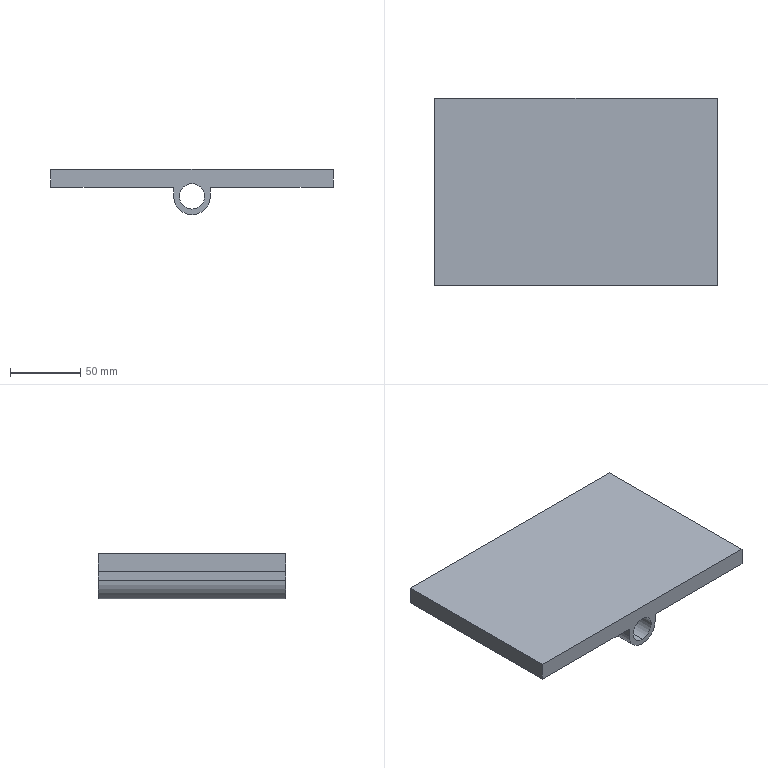Part | STEP file | 1 solid | 12 faces | box 200.887 x 133 x 32.213 mm | volume 365729 mm3 | plane 9 | cylinder 3 | commonest cylinder face diameters 18 x2 26.062 x1
STEP:
#1=CARTESIAN_POINT('',(0.,0.,0.));
#2=DIRECTION('',(0.,0.,1.));
#3=DIRECTION('',(1.,0.,0.));
#4=AXIS2_PLACEMENT_3D('',#1,#2,#3);
#5=CARTESIAN_POINT('',(340.649,394.014,170.933));
#6=VERTEX_POINT('',#5);
#7=CARTESIAN_POINT('',(340.649,527.014,170.933));
#8=VERTEX_POINT('',#7);
#9=CARTESIAN_POINT('',(340.649,394.014,170.933));
#10=DIRECTION('',(0.,1.,0.));
#11=VECTOR('',#10,1.);
#12=LINE('',#9,#11);
#13=CARTESIAN_POINT('',(340.649,394.014,161.933));
#14=DIRECTION('',(0.,1.,0.));
#15=DIRECTION('',(0.,0.,1.));
#16=AXIS2_PLACEMENT_3D('',#13,#14,#15);
#17=CYLINDRICAL_SURFACE('',#16,9.);
#18=CARTESIAN_POINT('',(6.283,0.));
#19=DIRECTION('',(0.,1.));
#20=VECTOR('',#19,1.);
#21=LINE('',#18,#20);
#22=(GEOMETRIC_REPRESENTATION_CONTEXT(2)PARAMETRIC_REPRESENTATION_CONTEXT()REPRESENTATION_CONTEXT('',''));
#23=DEFINITIONAL_REPRESENTATION('',(#21),#22);
#24=PCURVE('',#17,#23);
#25=CARTESIAN_POINT('',(340.649,394.014,161.933));
#26=DIRECTION('',(0.,1.,0.));
#27=DIRECTION('',(0.,0.,1.));
#28=AXIS2_PLACEMENT_3D('',#25,#26,#27);
#29=CYLINDRICAL_SURFACE('',#28,9.);
#30=CARTESIAN_POINT('',(0.,0.));
#31=DIRECTION('',(0.,1.));
#32=VECTOR('',#31,1.);
#33=LINE('',#30,#32);
#34=(GEOMETRIC_REPRESENTATION_CONTEXT(2)PARAMETRIC_REPRESENTATION_CONTEXT()REPRESENTATION_CONTEXT('',''));
#35=DEFINITIONAL_REPRESENTATION('',(#33),#34);
#36=PCURVE('',#29,#35);
#37=SURFACE_CURVE('',#12,(#24,#36),.PCURVE_S1.);
#38=EDGE_CURVE('',#6,#8,#37,.T.);
#39=ORIENTED_EDGE('',*,*,#38,.T.);
#40=CARTESIAN_POINT('',(340.649,527.014,152.933));
#41=VERTEX_POINT('',#40);
#42=CARTESIAN_POINT('',(340.649,527.014,161.933));
#43=DIRECTION('',(0.,1.,0.));
#44=DIRECTION('',(0.,0.,1.));
#45=AXIS2_PLACEMENT_3D('',#42,#43,#44);
#46=CIRCLE('',#45,9.);
#47=CARTESIAN_POINT('',(0.,133.));
#48=DIRECTION('',(1.,0.));
#49=VECTOR('',#48,1.);
#50=LINE('',#47,#49);
#51=(GEOMETRIC_REPRESENTATION_CONTEXT(2)PARAMETRIC_REPRESENTATION_CONTEXT()REPRESENTATION_CONTEXT('',''));
#52=DEFINITIONAL_REPRESENTATION('',(#50),#51);
#53=PCURVE('',#17,#52);
#54=CARTESIAN_POINT('',(0.,527.014,0.));
#55=DIRECTION('',(0.,1.,0.));
#56=DIRECTION('',(0.,0.,1.));
#57=AXIS2_PLACEMENT_3D('',#54,#55,#56);
#58=PLANE('',#57);
#59=CARTESIAN_POINT('',(161.933,340.649));
#60=DIRECTION('',(1.,0.));
#61=AXIS2_PLACEMENT_2D('',#59,#60);
#62=CIRCLE('',#61,9.);
#63=(GEOMETRIC_REPRESENTATION_CONTEXT(2)PARAMETRIC_REPRESENTATION_CONTEXT()REPRESENTATION_CONTEXT('',''));
#64=DEFINITIONAL_REPRESENTATION('',(#62),#63);
#65=PCURVE('',#58,#64);
#66=SURFACE_CURVE('',#46,(#53,#65),.PCURVE_S1.);
#67=EDGE_CURVE('',#41,#8,#66,.T.);
#68=ORIENTED_EDGE('',*,*,#67,.F.);
#69=CARTESIAN_POINT('',(340.649,394.014,152.933));
#70=VERTEX_POINT('',#69);
#71=CARTESIAN_POINT('',(340.649,394.014,152.933));
#72=DIRECTION('',(0.,1.,0.));
#73=VECTOR('',#72,1.);
#74=LINE('',#71,#73);
#75=CARTESIAN_POINT('',(3.142,0.));
#76=DIRECTION('',(0.,1.));
#77=VECTOR('',#76,1.);
#78=LINE('',#75,#77);
#79=(GEOMETRIC_REPRESENTATION_CONTEXT(2)PARAMETRIC_REPRESENTATION_CONTEXT()REPRESENTATION_CONTEXT('',''));
#80=DEFINITIONAL_REPRESENTATION('',(#78),#79);
#81=PCURVE('',#17,#80);
#82=CARTESIAN_POINT('',(3.142,0.));
#83=DIRECTION('',(0.,1.));
#84=VECTOR('',#83,1.);
#85=LINE('',#82,#84);
#86=(GEOMETRIC_REPRESENTATION_CONTEXT(2)PARAMETRIC_REPRESENTATION_CONTEXT()REPRESENTATION_CONTEXT('',''));
#87=DEFINITIONAL_REPRESENTATION('',(#85),#86);
#88=PCURVE('',#29,#87);
#89=SURFACE_CURVE('',#74,(#81,#88),.PCURVE_S1.);
#90=EDGE_CURVE('',#70,#41,#89,.T.);
#91=ORIENTED_EDGE('',*,*,#90,.F.);
#92=CARTESIAN_POINT('',(340.649,394.014,161.933));
#93=DIRECTION('',(0.,1.,0.));
#94=DIRECTION('',(0.,0.,1.));
#95=AXIS2_PLACEMENT_3D('',#92,#93,#94);
#96=CIRCLE('',#95,9.);
#97=CARTESIAN_POINT('',(0.,0.));
#98=DIRECTION('',(1.,0.));
#99=VECTOR('',#98,1.);
#100=LINE('',#97,#99);
#101=(GEOMETRIC_REPRESENTATION_CONTEXT(2)PARAMETRIC_REPRESENTATION_CONTEXT()REPRESENTATION_CONTEXT('',''));
#102=DEFINITIONAL_REPRESENTATION('',(#100),#101);
#103=PCURVE('',#17,#102);
#104=CARTESIAN_POINT('',(0.,394.014,0.));
#105=DIRECTION('',(0.,1.,0.));
#106=DIRECTION('',(0.,0.,1.));
#107=AXIS2_PLACEMENT_3D('',#104,#105,#106);
#108=PLANE('',#107);
#109=CARTESIAN_POINT('',(161.933,340.649));
#110=DIRECTION('',(1.,0.));
#111=AXIS2_PLACEMENT_2D('',#109,#110);
#112=CIRCLE('',#111,9.);
#113=(GEOMETRIC_REPRESENTATION_CONTEXT(2)PARAMETRIC_REPRESENTATION_CONTEXT()REPRESENTATION_CONTEXT('',''));
#114=DEFINITIONAL_REPRESENTATION('',(#112),#113);
#115=PCURVE('',#108,#114);
#116=SURFACE_CURVE('',#96,(#103,#115),.PCURVE_S1.);
#117=EDGE_CURVE('',#70,#6,#116,.T.);
#118=ORIENTED_EDGE('',*,*,#117,.T.);
#119=EDGE_LOOP('',(#39,#68,#91,#118));
#120=FACE_BOUND('',#119,.F.);
#121=ADVANCED_FACE('',(#120),#17,.F.);
#122=CARTESIAN_POINT('',(240.205,527.014,168.316));
#123=VERTEX_POINT('',#122);
#124=CARTESIAN_POINT('',(240.205,527.014,181.115));
#125=VERTEX_POINT('',#124);
#126=CARTESIAN_POINT('',(240.205,527.014,0.));
#127=DIRECTION('',(0.,0.,1.));
#128=VECTOR('',#127,1.);
#129=LINE('',#126,#128);
#130=CARTESIAN_POINT('',(240.205,394.014,0.));
#131=DIRECTION('',(-1.,0.,0.));
#132=DIRECTION('',(0.,0.,1.));
#133=AXIS2_PLACEMENT_3D('',#130,#131,#132);
#134=PLANE('',#133);
#135=CARTESIAN_POINT('',(0.,133.));
#136=DIRECTION('',(1.,0.));
#137=VECTOR('',#136,1.);
#138=LINE('',#135,#137);
#139=(GEOMETRIC_REPRESENTATION_CONTEXT(2)PARAMETRIC_REPRESENTATION_CONTEXT()REPRESENTATION_CONTEXT('',''));
#140=DEFINITIONAL_REPRESENTATION('',(#138),#139);
#141=PCURVE('',#134,#140);
#142=CARTESIAN_POINT('',(0.,240.205));
#143=DIRECTION('',(1.,0.));
#144=VECTOR('',#143,1.);
#145=LINE('',#142,#144);
#146=(GEOMETRIC_REPRESENTATION_CONTEXT(2)PARAMETRIC_REPRESENTATION_CONTEXT()REPRESENTATION_CONTEXT('',''));
#147=DEFINITIONAL_REPRESENTATION('',(#145),#146);
#148=PCURVE('',#58,#147);
#149=SURFACE_CURVE('',#129,(#141,#148),.PCURVE_S1.);
#150=EDGE_CURVE('',#123,#125,#149,.T.);
#151=ORIENTED_EDGE('',*,*,#150,.F.);
#152=CARTESIAN_POINT('',(240.205,394.014,168.316));
#153=VERTEX_POINT('',#152);
#154=CARTESIAN_POINT('',(240.205,394.014,168.316));
#155=DIRECTION('',(0.,1.,0.));
#156=VECTOR('',#155,1.);
#157=LINE('',#154,#156);
#158=CARTESIAN_POINT('',(168.316,0.));
#159=DIRECTION('',(0.,1.));
#160=VECTOR('',#159,1.);
#161=LINE('',#158,#160);
#162=(GEOMETRIC_REPRESENTATION_CONTEXT(2)PARAMETRIC_REPRESENTATION_CONTEXT()REPRESENTATION_CONTEXT('',''));
#163=DEFINITIONAL_REPRESENTATION('',(#161),#162);
#164=PCURVE('',#134,#163);
#165=CARTESIAN_POINT('',(0.,394.014,168.316));
#166=DIRECTION('',(0.,0.,1.));
#167=DIRECTION('',(1.,0.,0.));
#168=AXIS2_PLACEMENT_3D('',#165,#166,#167);
#169=PLANE('',#168);
#170=CARTESIAN_POINT('',(240.205,0.));
#171=DIRECTION('',(0.,1.));
#172=VECTOR('',#171,1.);
#173=LINE('',#170,#172);
#174=(GEOMETRIC_REPRESENTATION_CONTEXT(2)PARAMETRIC_REPRESENTATION_CONTEXT()REPRESENTATION_CONTEXT('',''));
#175=DEFINITIONAL_REPRESENTATION('',(#173),#174);
#176=PCURVE('',#169,#175);
#177=SURFACE_CURVE('',#157,(#164,#176),.PCURVE_S1.);
#178=EDGE_CURVE('',#153,#123,#177,.T.);
#179=ORIENTED_EDGE('',*,*,#178,.F.);
#180=CARTESIAN_POINT('',(240.205,394.014,181.115));
#181=VERTEX_POINT('',#180);
#182=CARTESIAN_POINT('',(240.205,394.014,0.));
#183=DIRECTION('',(0.,0.,1.));
#184=VECTOR('',#183,1.);
#185=LINE('',#182,#184);
#186=CARTESIAN_POINT('',(0.,0.));
#187=DIRECTION('',(1.,0.));
#188=VECTOR('',#187,1.);
#189=LINE('',#186,#188);
#190=(GEOMETRIC_REPRESENTATION_CONTEXT(2)PARAMETRIC_REPRESENTATION_CONTEXT()REPRESENTATION_CONTEXT('',''));
#191=DEFINITIONAL_REPRESENTATION('',(#189),#190);
#192=PCURVE('',#134,#191);
#193=CARTESIAN_POINT('',(0.,240.205));
#194=DIRECTION('',(1.,0.));
#195=VECTOR('',#194,1.);
#196=LINE('',#193,#195);
#197=(GEOMETRIC_REPRESENTATION_CONTEXT(2)PARAMETRIC_REPRESENTATION_CONTEXT()REPRESENTATION_CONTEXT('',''));
#198=DEFINITIONAL_REPRESENTATION('',(#196),#197);
#199=PCURVE('',#108,#198);
#200=SURFACE_CURVE('',#185,(#192,#199),.PCURVE_S1.);
#201=EDGE_CURVE('',#153,#181,#200,.T.);
#202=ORIENTED_EDGE('',*,*,#201,.T.);
#203=CARTESIAN_POINT('',(240.205,394.014,181.115));
#204=DIRECTION('',(0.,1.,0.));
#205=VECTOR('',#204,1.);
#206=LINE('',#203,#205);
#207=CARTESIAN_POINT('',(181.115,0.));
#208=DIRECTION('',(0.,1.));
#209=VECTOR('',#208,1.);
#210=LINE('',#207,#209);
#211=(GEOMETRIC_REPRESENTATION_CONTEXT(2)PARAMETRIC_REPRESENTATION_CONTEXT()REPRESENTATION_CONTEXT('',''));
#212=DEFINITIONAL_REPRESENTATION('',(#210),#211);
#213=PCURVE('',#134,#212);
#214=CARTESIAN_POINT('',(0.,394.014,181.115));
#215=DIRECTION('',(0.,0.,1.));
#216=DIRECTION('',(1.,0.,0.));
#217=AXIS2_PLACEMENT_3D('',#214,#215,#216);
#218=PLANE('',#217);
#219=CARTESIAN_POINT('',(240.205,0.));
#220=DIRECTION('',(0.,1.));
#221=VECTOR('',#220,1.);
#222=LINE('',#219,#221);
#223=(GEOMETRIC_REPRESENTATION_CONTEXT(2)PARAMETRIC_REPRESENTATION_CONTEXT()REPRESENTATION_CONTEXT('',''));
#224=DEFINITIONAL_REPRESENTATION('',(#222),#223);
#225=PCURVE('',#218,#224);
#226=SURFACE_CURVE('',#206,(#213,#225),.PCURVE_S1.);
#227=EDGE_CURVE('',#181,#125,#226,.T.);
#228=ORIENTED_EDGE('',*,*,#227,.T.);
#229=EDGE_LOOP('',(#151,#179,#202,#228));
#230=FACE_BOUND('',#229,.T.);
#231=ADVANCED_FACE('',(#230),#134,.T.);
#232=CARTESIAN_POINT('',(327.618,527.014,168.316));
#233=VERTEX_POINT('',#232);
#234=CARTESIAN_POINT('',(0.,527.014,168.316));
#235=DIRECTION('',(1.,0.,0.));
#236=VECTOR('',#235,1.);
#237=LINE('',#234,#236);
#238=CARTESIAN_POINT('',(0.,133.));
#239=DIRECTION('',(1.,0.));
#240=VECTOR('',#239,1.);
#241=LINE('',#238,#240);
#242=(GEOMETRIC_REPRESENTATION_CONTEXT(2)PARAMETRIC_REPRESENTATION_CONTEXT()REPRESENTATION_CONTEXT('',''));
#243=DEFINITIONAL_REPRESENTATION('',(#241),#242);
#244=PCURVE('',#169,#243);
#245=CARTESIAN_POINT('',(168.316,0.));
#246=DIRECTION('',(0.,1.));
#247=VECTOR('',#246,1.);
#248=LINE('',#245,#247);
#249=(GEOMETRIC_REPRESENTATION_CONTEXT(2)PARAMETRIC_REPRESENTATION_CONTEXT()REPRESENTATION_CONTEXT('',''));
#250=DEFINITIONAL_REPRESENTATION('',(#248),#249);
#251=PCURVE('',#58,#250);
#252=SURFACE_CURVE('',#237,(#244,#251),.PCURVE_S1.);
#253=EDGE_CURVE('',#123,#233,#252,.T.);
#254=ORIENTED_EDGE('',*,*,#253,.T.);
#255=CARTESIAN_POINT('',(327.618,394.014,168.316));
#256=VERTEX_POINT('',#255);
#257=CARTESIAN_POINT('',(327.618,394.014,168.316));
#258=DIRECTION('',(0.,1.,0.));
#259=VECTOR('',#258,1.);
#260=LINE('',#257,#259);
#261=CARTESIAN_POINT('',(327.618,0.));
#262=DIRECTION('',(0.,1.));
#263=VECTOR('',#262,1.);
#264=LINE('',#261,#263);
#265=(GEOMETRIC_REPRESENTATION_CONTEXT(2)PARAMETRIC_REPRESENTATION_CONTEXT()REPRESENTATION_CONTEXT('',''));
#266=DEFINITIONAL_REPRESENTATION('',(#264),#265);
#267=PCURVE('',#169,#266);
#268=CARTESIAN_POINT('',(327.618,394.014,0.));
#269=DIRECTION('',(-1.,0.,0.));
#270=DIRECTION('',(0.,0.,1.));
#271=AXIS2_PLACEMENT_3D('',#268,#269,#270);
#272=PLANE('',#271);
#273=CARTESIAN_POINT('',(168.316,0.));
#274=DIRECTION('',(0.,1.));
#275=VECTOR('',#274,1.);
#276=LINE('',#273,#275);
#277=(GEOMETRIC_REPRESENTATION_CONTEXT(2)PARAMETRIC_REPRESENTATION_CONTEXT()REPRESENTATION_CONTEXT('',''));
#278=DEFINITIONAL_REPRESENTATION('',(#276),#277);
#279=PCURVE('',#272,#278);
#280=SURFACE_CURVE('',#260,(#267,#279),.PCURVE_S1.);
#281=EDGE_CURVE('',#256,#233,#280,.T.);
#282=ORIENTED_EDGE('',*,*,#281,.F.);
#283=CARTESIAN_POINT('',(0.,394.014,168.316));
#284=DIRECTION('',(1.,0.,0.));
#285=VECTOR('',#284,1.);
#286=LINE('',#283,#285);
#287=CARTESIAN_POINT('',(0.,0.));
#288=DIRECTION('',(1.,0.));
#289=VECTOR('',#288,1.);
#290=LINE('',#287,#289);
#291=(GEOMETRIC_REPRESENTATION_CONTEXT(2)PARAMETRIC_REPRESENTATION_CONTEXT()REPRESENTATION_CONTEXT('',''));
#292=DEFINITIONAL_REPRESENTATION('',(#290),#291);
#293=PCURVE('',#169,#292);
#294=CARTESIAN_POINT('',(168.316,0.));
#295=DIRECTION('',(0.,1.));
#296=VECTOR('',#295,1.);
#297=LINE('',#294,#296);
#298=(GEOMETRIC_REPRESENTATION_CONTEXT(2)PARAMETRIC_REPRESENTATION_CONTEXT()REPRESENTATION_CONTEXT('',''));
#299=DEFINITIONAL_REPRESENTATION('',(#297),#298);
#300=PCURVE('',#108,#299);
#301=SURFACE_CURVE('',#286,(#293,#300),.PCURVE_S1.);
#302=EDGE_CURVE('',#153,#256,#301,.T.);
#303=ORIENTED_EDGE('',*,*,#302,.F.);
#304=ORIENTED_EDGE('',*,*,#178,.T.);
#305=EDGE_LOOP('',(#254,#282,#303,#304));
#306=FACE_BOUND('',#305,.T.);
#307=ADVANCED_FACE('',(#306),#169,.F.);
#308=CARTESIAN_POINT('',(327.618,527.014,161.933));
#309=VERTEX_POINT('',#308);
#310=CARTESIAN_POINT('',(327.618,527.014,0.));
#311=DIRECTION('',(0.,0.,1.));
#312=VECTOR('',#311,1.);
#313=LINE('',#310,#312);
#314=CARTESIAN_POINT('',(0.,133.));
#315=DIRECTION('',(1.,0.));
#316=VECTOR('',#315,1.);
#317=LINE('',#314,#316);
#318=(GEOMETRIC_REPRESENTATION_CONTEXT(2)PARAMETRIC_REPRESENTATION_CONTEXT()REPRESENTATION_CONTEXT('',''));
#319=DEFINITIONAL_REPRESENTATION('',(#317),#318);
#320=PCURVE('',#272,#319);
#321=CARTESIAN_POINT('',(0.,327.618));
#322=DIRECTION('',(1.,0.));
#323=VECTOR('',#322,1.);
#324=LINE('',#321,#323);
#325=(GEOMETRIC_REPRESENTATION_CONTEXT(2)PARAMETRIC_REPRESENTATION_CONTEXT()REPRESENTATION_CONTEXT('',''));
#326=DEFINITIONAL_REPRESENTATION('',(#324),#325);
#327=PCURVE('',#58,#326);
#328=SURFACE_CURVE('',#313,(#320,#327),.PCURVE_S1.);
#329=EDGE_CURVE('',#309,#233,#328,.T.);
#330=ORIENTED_EDGE('',*,*,#329,.F.);
#331=CARTESIAN_POINT('',(327.618,394.014,161.933));
#332=VERTEX_POINT('',#331);
#333=CARTESIAN_POINT('',(327.618,394.014,161.933));
#334=DIRECTION('',(0.,1.,0.));
#335=VECTOR('',#334,1.);
#336=LINE('',#333,#335);
#337=CARTESIAN_POINT('',(161.933,0.));
#338=DIRECTION('',(0.,1.));
#339=VECTOR('',#338,1.);
#340=LINE('',#337,#339);
#341=(GEOMETRIC_REPRESENTATION_CONTEXT(2)PARAMETRIC_REPRESENTATION_CONTEXT()REPRESENTATION_CONTEXT('',''));
#342=DEFINITIONAL_REPRESENTATION('',(#340),#341);
#343=PCURVE('',#272,#342);
#344=CARTESIAN_POINT('',(340.649,394.014,161.933));
#345=DIRECTION('',(0.,1.,0.));
#346=DIRECTION('',(0.,0.,1.));
#347=AXIS2_PLACEMENT_3D('',#344,#345,#346);
#348=CYLINDRICAL_SURFACE('',#347,13.031);
#349=CARTESIAN_POINT('',(4.712,0.));
#350=DIRECTION('',(0.,1.));
#351=VECTOR('',#350,1.);
#352=LINE('',#349,#351);
#353=(GEOMETRIC_REPRESENTATION_CONTEXT(2)PARAMETRIC_REPRESENTATION_CONTEXT()REPRESENTATION_CONTEXT('',''));
#354=DEFINITIONAL_REPRESENTATION('',(#352),#353);
#355=PCURVE('',#348,#354);
#356=SURFACE_CURVE('',#336,(#343,#355),.PCURVE_S1.);
#357=EDGE_CURVE('',#332,#309,#356,.T.);
#358=ORIENTED_EDGE('',*,*,#357,.F.);
#359=CARTESIAN_POINT('',(327.618,394.014,0.));
#360=DIRECTION('',(0.,0.,1.));
#361=VECTOR('',#360,1.);
#362=LINE('',#359,#361);
#363=CARTESIAN_POINT('',(0.,0.));
#364=DIRECTION('',(1.,0.));
#365=VECTOR('',#364,1.);
#366=LINE('',#363,#365);
#367=(GEOMETRIC_REPRESENTATION_CONTEXT(2)PARAMETRIC_REPRESENTATION_CONTEXT()REPRESENTATION_CONTEXT('',''));
#368=DEFINITIONAL_REPRESENTATION('',(#366),#367);
#369=PCURVE('',#272,#368);
#370=CARTESIAN_POINT('',(0.,327.618));
#371=DIRECTION('',(1.,0.));
#372=VECTOR('',#371,1.);
#373=LINE('',#370,#372);
#374=(GEOMETRIC_REPRESENTATION_CONTEXT(2)PARAMETRIC_REPRESENTATION_CONTEXT()REPRESENTATION_CONTEXT('',''));
#375=DEFINITIONAL_REPRESENTATION('',(#373),#374);
#376=PCURVE('',#108,#375);
#377=SURFACE_CURVE('',#362,(#369,#376),.PCURVE_S1.);
#378=EDGE_CURVE('',#332,#256,#377,.T.);
#379=ORIENTED_EDGE('',*,*,#378,.T.);
#380=ORIENTED_EDGE('',*,*,#281,.T.);
#381=EDGE_LOOP('',(#330,#358,#379,#380));
#382=FACE_BOUND('',#381,.T.);
#383=ADVANCED_FACE('',(#382),#272,.T.);
#384=CARTESIAN_POINT('',(353.68,527.014,161.933));
#385=VERTEX_POINT('',#384);
#386=CARTESIAN_POINT('',(340.649,527.014,161.933));
#387=DIRECTION('',(0.,1.,0.));
#388=DIRECTION('',(0.,0.,1.));
#389=AXIS2_PLACEMENT_3D('',#386,#387,#388);
#390=CIRCLE('',#389,13.031);
#391=CARTESIAN_POINT('',(0.,133.));
#392=DIRECTION('',(1.,0.));
#393=VECTOR('',#392,1.);
#394=LINE('',#391,#393);
#395=(GEOMETRIC_REPRESENTATION_CONTEXT(2)PARAMETRIC_REPRESENTATION_CONTEXT()REPRESENTATION_CONTEXT('',''));
#396=DEFINITIONAL_REPRESENTATION('',(#394),#395);
#397=PCURVE('',#348,#396);
#398=CARTESIAN_POINT('',(161.933,340.649));
#399=DIRECTION('',(1.,0.));
#400=AXIS2_PLACEMENT_2D('',#398,#399);
#401=CIRCLE('',#400,13.031);
#402=(GEOMETRIC_REPRESENTATION_CONTEXT(2)PARAMETRIC_REPRESENTATION_CONTEXT()REPRESENTATION_CONTEXT('',''));
#403=DEFINITIONAL_REPRESENTATION('',(#401),#402);
#404=PCURVE('',#58,#403);
#405=SURFACE_CURVE('',#390,(#397,#404),.PCURVE_S1.);
#406=EDGE_CURVE('',#385,#309,#405,.T.);
#407=ORIENTED_EDGE('',*,*,#406,.F.);
#408=CARTESIAN_POINT('',(353.68,394.014,161.933));
#409=VERTEX_POINT('',#408);
#410=CARTESIAN_POINT('',(353.68,394.014,161.933));
#411=DIRECTION('',(0.,1.,0.));
#412=VECTOR('',#411,1.);
#413=LINE('',#410,#412);
#414=CARTESIAN_POINT('',(1.571,0.));
#415=DIRECTION('',(0.,1.));
#416=VECTOR('',#415,1.);
#417=LINE('',#414,#416);
#418=(GEOMETRIC_REPRESENTATION_CONTEXT(2)PARAMETRIC_REPRESENTATION_CONTEXT()REPRESENTATION_CONTEXT('',''));
#419=DEFINITIONAL_REPRESENTATION('',(#417),#418);
#420=PCURVE('',#348,#419);
#421=CARTESIAN_POINT('',(353.68,394.014,0.));
#422=DIRECTION('',(-1.,0.,0.));
#423=DIRECTION('',(0.,0.,1.));
#424=AXIS2_PLACEMENT_3D('',#421,#422,#423);
#425=PLANE('',#424);
#426=CARTESIAN_POINT('',(161.933,0.));
#427=DIRECTION('',(0.,1.));
#428=VECTOR('',#427,1.);
#429=LINE('',#426,#428);
#430=(GEOMETRIC_REPRESENTATION_CONTEXT(2)PARAMETRIC_REPRESENTATION_CONTEXT()REPRESENTATION_CONTEXT('',''));
#431=DEFINITIONAL_REPRESENTATION('',(#429),#430);
#432=PCURVE('',#425,#431);
#433=SURFACE_CURVE('',#413,(#420,#432),.PCURVE_S1.);
#434=EDGE_CURVE('',#409,#385,#433,.T.);
#435=ORIENTED_EDGE('',*,*,#434,.F.);
#436=CARTESIAN_POINT('',(340.649,394.014,161.933));
#437=DIRECTION('',(0.,1.,0.));
#438=DIRECTION('',(0.,0.,1.));
#439=AXIS2_PLACEMENT_3D('',#436,#437,#438);
#440=CIRCLE('',#439,13.031);
#441=CARTESIAN_POINT('',(0.,0.));
#442=DIRECTION('',(1.,0.));
#443=VECTOR('',#442,1.);
#444=LINE('',#441,#443);
#445=(GEOMETRIC_REPRESENTATION_CONTEXT(2)PARAMETRIC_REPRESENTATION_CONTEXT()REPRESENTATION_CONTEXT('',''));
#446=DEFINITIONAL_REPRESENTATION('',(#444),#445);
#447=PCURVE('',#348,#446);
#448=CARTESIAN_POINT('',(161.933,340.649));
#449=DIRECTION('',(1.,0.));
#450=AXIS2_PLACEMENT_2D('',#448,#449);
#451=CIRCLE('',#450,13.031);
#452=(GEOMETRIC_REPRESENTATION_CONTEXT(2)PARAMETRIC_REPRESENTATION_CONTEXT()REPRESENTATION_CONTEXT('',''));
#453=DEFINITIONAL_REPRESENTATION('',(#451),#452);
#454=PCURVE('',#108,#453);
#455=SURFACE_CURVE('',#440,(#447,#454),.PCURVE_S1.);
#456=EDGE_CURVE('',#409,#332,#455,.T.);
#457=ORIENTED_EDGE('',*,*,#456,.T.);
#458=ORIENTED_EDGE('',*,*,#357,.T.);
#459=EDGE_LOOP('',(#407,#435,#457,#458));
#460=FACE_BOUND('',#459,.T.);
#461=ADVANCED_FACE('',(#460),#348,.T.);
#462=CARTESIAN_POINT('',(353.68,527.014,168.316));
#463=VERTEX_POINT('',#462);
#464=CARTESIAN_POINT('',(353.68,527.014,0.));
#465=DIRECTION('',(0.,0.,1.));
#466=VECTOR('',#465,1.);
#467=LINE('',#464,#466);
#468=CARTESIAN_POINT('',(0.,133.));
#469=DIRECTION('',(1.,0.));
#470=VECTOR('',#469,1.);
#471=LINE('',#468,#470);
#472=(GEOMETRIC_REPRESENTATION_CONTEXT(2)PARAMETRIC_REPRESENTATION_CONTEXT()REPRESENTATION_CONTEXT('',''));
#473=DEFINITIONAL_REPRESENTATION('',(#471),#472);
#474=PCURVE('',#425,#473);
#475=CARTESIAN_POINT('',(0.,353.68));
#476=DIRECTION('',(1.,0.));
#477=VECTOR('',#476,1.);
#478=LINE('',#475,#477);
#479=(GEOMETRIC_REPRESENTATION_CONTEXT(2)PARAMETRIC_REPRESENTATION_CONTEXT()REPRESENTATION_CONTEXT('',''));
#480=DEFINITIONAL_REPRESENTATION('',(#478),#479);
#481=PCURVE('',#58,#480);
#482=SURFACE_CURVE('',#467,(#474,#481),.PCURVE_S1.);
#483=EDGE_CURVE('',#385,#463,#482,.T.);
#484=ORIENTED_EDGE('',*,*,#483,.T.);
#485=CARTESIAN_POINT('',(353.68,394.014,168.316));
#486=VERTEX_POINT('',#485);
#487=CARTESIAN_POINT('',(353.68,394.014,168.316));
#488=DIRECTION('',(0.,1.,0.));
#489=VECTOR('',#488,1.);
#490=LINE('',#487,#489);
#491=CARTESIAN_POINT('',(168.316,0.));
#492=DIRECTION('',(0.,1.));
#493=VECTOR('',#492,1.);
#494=LINE('',#491,#493);
#495=(GEOMETRIC_REPRESENTATION_CONTEXT(2)PARAMETRIC_REPRESENTATION_CONTEXT()REPRESENTATION_CONTEXT('',''));
#496=DEFINITIONAL_REPRESENTATION('',(#494),#495);
#497=PCURVE('',#425,#496);
#498=CARTESIAN_POINT('',(0.,394.014,168.316));
#499=DIRECTION('',(0.,0.,1.));
#500=DIRECTION('',(1.,0.,0.));
#501=AXIS2_PLACEMENT_3D('',#498,#499,#500);
#502=PLANE('',#501);
#503=CARTESIAN_POINT('',(353.68,0.));
#504=DIRECTION('',(0.,1.));
#505=VECTOR('',#504,1.);
#506=LINE('',#503,#505);
#507=(GEOMETRIC_REPRESENTATION_CONTEXT(2)PARAMETRIC_REPRESENTATION_CONTEXT()REPRESENTATION_CONTEXT('',''));
#508=DEFINITIONAL_REPRESENTATION('',(#506),#507);
#509=PCURVE('',#502,#508);
#510=SURFACE_CURVE('',#490,(#497,#509),.PCURVE_S1.);
#511=EDGE_CURVE('',#486,#463,#510,.T.);
#512=ORIENTED_EDGE('',*,*,#511,.F.);
#513=CARTESIAN_POINT('',(353.68,394.014,0.));
#514=DIRECTION('',(0.,0.,1.));
#515=VECTOR('',#514,1.);
#516=LINE('',#513,#515);
#517=CARTESIAN_POINT('',(0.,0.));
#518=DIRECTION('',(1.,0.));
#519=VECTOR('',#518,1.);
#520=LINE('',#517,#519);
#521=(GEOMETRIC_REPRESENTATION_CONTEXT(2)PARAMETRIC_REPRESENTATION_CONTEXT()REPRESENTATION_CONTEXT('',''));
#522=DEFINITIONAL_REPRESENTATION('',(#520),#521);
#523=PCURVE('',#425,#522);
#524=CARTESIAN_POINT('',(0.,353.68));
#525=DIRECTION('',(1.,0.));
#526=VECTOR('',#525,1.);
#527=LINE('',#524,#526);
#528=(GEOMETRIC_REPRESENTATION_CONTEXT(2)PARAMETRIC_REPRESENTATION_CONTEXT()REPRESENTATION_CONTEXT('',''));
#529=DEFINITIONAL_REPRESENTATION('',(#527),#528);
#530=PCURVE('',#108,#529);
#531=SURFACE_CURVE('',#516,(#523,#530),.PCURVE_S1.);
#532=EDGE_CURVE('',#409,#486,#531,.T.);
#533=ORIENTED_EDGE('',*,*,#532,.F.);
#534=ORIENTED_EDGE('',*,*,#434,.T.);
#535=EDGE_LOOP('',(#484,#512,#533,#534));
#536=FACE_BOUND('',#535,.T.);
#537=ADVANCED_FACE('',(#536),#425,.F.);
#538=CARTESIAN_POINT('',(441.092,527.014,168.316));
#539=VERTEX_POINT('',#538);
#540=CARTESIAN_POINT('',(0.,527.014,168.316));
#541=DIRECTION('',(1.,0.,0.));
#542=VECTOR('',#541,1.);
#543=LINE('',#540,#542);
#544=CARTESIAN_POINT('',(0.,133.));
#545=DIRECTION('',(1.,0.));
#546=VECTOR('',#545,1.);
#547=LINE('',#544,#546);
#548=(GEOMETRIC_REPRESENTATION_CONTEXT(2)PARAMETRIC_REPRESENTATION_CONTEXT()REPRESENTATION_CONTEXT('',''));
#549=DEFINITIONAL_REPRESENTATION('',(#547),#548);
#550=PCURVE('',#502,#549);
#551=CARTESIAN_POINT('',(168.316,0.));
#552=DIRECTION('',(0.,1.));
#553=VECTOR('',#552,1.);
#554=LINE('',#551,#553);
#555=(GEOMETRIC_REPRESENTATION_CONTEXT(2)PARAMETRIC_REPRESENTATION_CONTEXT()REPRESENTATION_CONTEXT('',''));
#556=DEFINITIONAL_REPRESENTATION('',(#554),#555);
#557=PCURVE('',#58,#556);
#558=SURFACE_CURVE('',#543,(#550,#557),.PCURVE_S1.);
#559=EDGE_CURVE('',#463,#539,#558,.T.);
#560=ORIENTED_EDGE('',*,*,#559,.T.);
#561=CARTESIAN_POINT('',(441.092,394.014,168.316));
#562=VERTEX_POINT('',#561);
#563=CARTESIAN_POINT('',(441.092,394.014,168.316));
#564=DIRECTION('',(0.,1.,0.));
#565=VECTOR('',#564,1.);
#566=LINE('',#563,#565);
#567=CARTESIAN_POINT('',(441.092,0.));
#568=DIRECTION('',(0.,1.));
#569=VECTOR('',#568,1.);
#570=LINE('',#567,#569);
#571=(GEOMETRIC_REPRESENTATION_CONTEXT(2)PARAMETRIC_REPRESENTATION_CONTEXT()REPRESENTATION_CONTEXT('',''));
#572=DEFINITIONAL_REPRESENTATION('',(#570),#571);
#573=PCURVE('',#502,#572);
#574=CARTESIAN_POINT('',(441.092,394.014,0.));
#575=DIRECTION('',(-1.,0.,0.));
#576=DIRECTION('',(0.,0.,1.));
#577=AXIS2_PLACEMENT_3D('',#574,#575,#576);
#578=PLANE('',#577);
#579=CARTESIAN_POINT('',(168.316,0.));
#580=DIRECTION('',(0.,1.));
#581=VECTOR('',#580,1.);
#582=LINE('',#579,#581);
#583=(GEOMETRIC_REPRESENTATION_CONTEXT(2)PARAMETRIC_REPRESENTATION_CONTEXT()REPRESENTATION_CONTEXT('',''));
#584=DEFINITIONAL_REPRESENTATION('',(#582),#583);
#585=PCURVE('',#578,#584);
#586=SURFACE_CURVE('',#566,(#573,#585),.PCURVE_S1.);
#587=EDGE_CURVE('',#562,#539,#586,.T.);
#588=ORIENTED_EDGE('',*,*,#587,.F.);
#589=CARTESIAN_POINT('',(0.,394.014,168.316));
#590=DIRECTION('',(1.,0.,0.));
#591=VECTOR('',#590,1.);
#592=LINE('',#589,#591);
#593=CARTESIAN_POINT('',(0.,0.));
#594=DIRECTION('',(1.,0.));
#595=VECTOR('',#594,1.);
#596=LINE('',#593,#595);
#597=(GEOMETRIC_REPRESENTATION_CONTEXT(2)PARAMETRIC_REPRESENTATION_CONTEXT()REPRESENTATION_CONTEXT('',''));
#598=DEFINITIONAL_REPRESENTATION('',(#596),#597);
#599=PCURVE('',#502,#598);
#600=CARTESIAN_POINT('',(168.316,0.));
#601=DIRECTION('',(0.,1.));
#602=VECTOR('',#601,1.);
#603=LINE('',#600,#602);
#604=(GEOMETRIC_REPRESENTATION_CONTEXT(2)PARAMETRIC_REPRESENTATION_CONTEXT()REPRESENTATION_CONTEXT('',''));
#605=DEFINITIONAL_REPRESENTATION('',(#603),#604);
#606=PCURVE('',#108,#605);
#607=SURFACE_CURVE('',#592,(#599,#606),.PCURVE_S1.);
#608=EDGE_CURVE('',#486,#562,#607,.T.);
#609=ORIENTED_EDGE('',*,*,#608,.F.);
#610=ORIENTED_EDGE('',*,*,#511,.T.);
#611=EDGE_LOOP('',(#560,#588,#609,#610));
#612=FACE_BOUND('',#611,.T.);
#613=ADVANCED_FACE('',(#612),#502,.F.);
#614=CARTESIAN_POINT('',(441.092,527.014,181.115));
#615=VERTEX_POINT('',#614);
#616=CARTESIAN_POINT('',(441.092,527.014,0.));
#617=DIRECTION('',(0.,0.,1.));
#618=VECTOR('',#617,1.);
#619=LINE('',#616,#618);
#620=CARTESIAN_POINT('',(0.,133.));
#621=DIRECTION('',(1.,0.));
#622=VECTOR('',#621,1.);
#623=LINE('',#620,#622);
#624=(GEOMETRIC_REPRESENTATION_CONTEXT(2)PARAMETRIC_REPRESENTATION_CONTEXT()REPRESENTATION_CONTEXT('',''));
#625=DEFINITIONAL_REPRESENTATION('',(#623),#624);
#626=PCURVE('',#578,#625);
#627=CARTESIAN_POINT('',(0.,441.092));
#628=DIRECTION('',(1.,0.));
#629=VECTOR('',#628,1.);
#630=LINE('',#627,#629);
#631=(GEOMETRIC_REPRESENTATION_CONTEXT(2)PARAMETRIC_REPRESENTATION_CONTEXT()REPRESENTATION_CONTEXT('',''));
#632=DEFINITIONAL_REPRESENTATION('',(#630),#631);
#633=PCURVE('',#58,#632);
#634=SURFACE_CURVE('',#619,(#626,#633),.PCURVE_S1.);
#635=EDGE_CURVE('',#539,#615,#634,.T.);
#636=ORIENTED_EDGE('',*,*,#635,.T.);
#637=CARTESIAN_POINT('',(441.092,394.014,181.115));
#638=VERTEX_POINT('',#637);
#639=CARTESIAN_POINT('',(441.092,394.014,181.115));
#640=DIRECTION('',(0.,1.,0.));
#641=VECTOR('',#640,1.);
#642=LINE('',#639,#641);
#643=CARTESIAN_POINT('',(181.115,0.));
#644=DIRECTION('',(0.,1.));
#645=VECTOR('',#644,1.);
#646=LINE('',#643,#645);
#647=(GEOMETRIC_REPRESENTATION_CONTEXT(2)PARAMETRIC_REPRESENTATION_CONTEXT()REPRESENTATION_CONTEXT('',''));
#648=DEFINITIONAL_REPRESENTATION('',(#646),#647);
#649=PCURVE('',#578,#648);
#650=CARTESIAN_POINT('',(441.092,0.));
#651=DIRECTION('',(0.,1.));
#652=VECTOR('',#651,1.);
#653=LINE('',#650,#652);
#654=(GEOMETRIC_REPRESENTATION_CONTEXT(2)PARAMETRIC_REPRESENTATION_CONTEXT()REPRESENTATION_CONTEXT('',''));
#655=DEFINITIONAL_REPRESENTATION('',(#653),#654);
#656=PCURVE('',#218,#655);
#657=SURFACE_CURVE('',#642,(#649,#656),.PCURVE_S1.);
#658=EDGE_CURVE('',#638,#615,#657,.T.);
#659=ORIENTED_EDGE('',*,*,#658,.F.);
#660=CARTESIAN_POINT('',(441.092,394.014,0.));
#661=DIRECTION('',(0.,0.,1.));
#662=VECTOR('',#661,1.);
#663=LINE('',#660,#662);
#664=CARTESIAN_POINT('',(0.,0.));
#665=DIRECTION('',(1.,0.));
#666=VECTOR('',#665,1.);
#667=LINE('',#664,#666);
#668=(GEOMETRIC_REPRESENTATION_CONTEXT(2)PARAMETRIC_REPRESENTATION_CONTEXT()REPRESENTATION_CONTEXT('',''));
#669=DEFINITIONAL_REPRESENTATION('',(#667),#668);
#670=PCURVE('',#578,#669);
#671=CARTESIAN_POINT('',(0.,441.092));
#672=DIRECTION('',(1.,0.));
#673=VECTOR('',#672,1.);
#674=LINE('',#671,#673);
#675=(GEOMETRIC_REPRESENTATION_CONTEXT(2)PARAMETRIC_REPRESENTATION_CONTEXT()REPRESENTATION_CONTEXT('',''));
#676=DEFINITIONAL_REPRESENTATION('',(#674),#675);
#677=PCURVE('',#108,#676);
#678=SURFACE_CURVE('',#663,(#670,#677),.PCURVE_S1.);
#679=EDGE_CURVE('',#562,#638,#678,.T.);
#680=ORIENTED_EDGE('',*,*,#679,.F.);
#681=ORIENTED_EDGE('',*,*,#587,.T.);
#682=EDGE_LOOP('',(#636,#659,#680,#681));
#683=FACE_BOUND('',#682,.T.);
#684=ADVANCED_FACE('',(#683),#578,.F.);
#685=CARTESIAN_POINT('',(0.,527.014,181.115));
#686=DIRECTION('',(1.,0.,0.));
#687=VECTOR('',#686,1.);
#688=LINE('',#685,#687);
#689=CARTESIAN_POINT('',(0.,133.));
#690=DIRECTION('',(1.,0.));
#691=VECTOR('',#690,1.);
#692=LINE('',#689,#691);
#693=(GEOMETRIC_REPRESENTATION_CONTEXT(2)PARAMETRIC_REPRESENTATION_CONTEXT()REPRESENTATION_CONTEXT('',''));
#694=DEFINITIONAL_REPRESENTATION('',(#692),#693);
#695=PCURVE('',#218,#694);
#696=CARTESIAN_POINT('',(181.115,0.));
#697=DIRECTION('',(0.,1.));
#698=VECTOR('',#697,1.);
#699=LINE('',#696,#698);
#700=(GEOMETRIC_REPRESENTATION_CONTEXT(2)PARAMETRIC_REPRESENTATION_CONTEXT()REPRESENTATION_CONTEXT('',''));
#701=DEFINITIONAL_REPRESENTATION('',(#699),#700);
#702=PCURVE('',#58,#701);
#703=SURFACE_CURVE('',#688,(#695,#702),.PCURVE_S1.);
#704=EDGE_CURVE('',#125,#615,#703,.T.);
#705=ORIENTED_EDGE('',*,*,#704,.F.);
#706=ORIENTED_EDGE('',*,*,#227,.F.);
#707=CARTESIAN_POINT('',(0.,394.014,181.115));
#708=DIRECTION('',(1.,0.,0.));
#709=VECTOR('',#708,1.);
#710=LINE('',#707,#709);
#711=CARTESIAN_POINT('',(0.,0.));
#712=DIRECTION('',(1.,0.));
#713=VECTOR('',#712,1.);
#714=LINE('',#711,#713);
#715=(GEOMETRIC_REPRESENTATION_CONTEXT(2)PARAMETRIC_REPRESENTATION_CONTEXT()REPRESENTATION_CONTEXT('',''));
#716=DEFINITIONAL_REPRESENTATION('',(#714),#715);
#717=PCURVE('',#218,#716);
#718=CARTESIAN_POINT('',(181.115,0.));
#719=DIRECTION('',(0.,1.));
#720=VECTOR('',#719,1.);
#721=LINE('',#718,#720);
#722=(GEOMETRIC_REPRESENTATION_CONTEXT(2)PARAMETRIC_REPRESENTATION_CONTEXT()REPRESENTATION_CONTEXT('',''));
#723=DEFINITIONAL_REPRESENTATION('',(#721),#722);
#724=PCURVE('',#108,#723);
#725=SURFACE_CURVE('',#710,(#717,#724),.PCURVE_S1.);
#726=EDGE_CURVE('',#181,#638,#725,.T.);
#727=ORIENTED_EDGE('',*,*,#726,.T.);
#728=ORIENTED_EDGE('',*,*,#658,.T.);
#729=EDGE_LOOP('',(#705,#706,#727,#728));
#730=FACE_BOUND('',#729,.T.);
#731=ADVANCED_FACE('',(#730),#218,.T.);
#732=CARTESIAN_POINT('',(340.649,527.014,161.933));
#733=DIRECTION('',(0.,1.,0.));
#734=DIRECTION('',(0.,0.,1.));
#735=AXIS2_PLACEMENT_3D('',#732,#733,#734);
#736=CIRCLE('',#735,9.);
#737=CARTESIAN_POINT('',(0.,133.));
#738=DIRECTION('',(1.,0.));
#739=VECTOR('',#738,1.);
#740=LINE('',#737,#739);
#741=(GEOMETRIC_REPRESENTATION_CONTEXT(2)PARAMETRIC_REPRESENTATION_CONTEXT()REPRESENTATION_CONTEXT('',''));
#742=DEFINITIONAL_REPRESENTATION('',(#740),#741);
#743=PCURVE('',#29,#742);
#744=CARTESIAN_POINT('',(161.933,340.649));
#745=DIRECTION('',(1.,0.));
#746=AXIS2_PLACEMENT_2D('',#744,#745);
#747=CIRCLE('',#746,9.);
#748=(GEOMETRIC_REPRESENTATION_CONTEXT(2)PARAMETRIC_REPRESENTATION_CONTEXT()REPRESENTATION_CONTEXT('',''));
#749=DEFINITIONAL_REPRESENTATION('',(#747),#748);
#750=PCURVE('',#58,#749);
#751=SURFACE_CURVE('',#736,(#743,#750),.PCURVE_S1.);
#752=EDGE_CURVE('',#8,#41,#751,.T.);
#753=ORIENTED_EDGE('',*,*,#752,.F.);
#754=ORIENTED_EDGE('',*,*,#38,.F.);
#755=CARTESIAN_POINT('',(340.649,394.014,161.933));
#756=DIRECTION('',(0.,1.,0.));
#757=DIRECTION('',(0.,0.,1.));
#758=AXIS2_PLACEMENT_3D('',#755,#756,#757);
#759=CIRCLE('',#758,9.);
#760=CARTESIAN_POINT('',(0.,0.));
#761=DIRECTION('',(1.,0.));
#762=VECTOR('',#761,1.);
#763=LINE('',#760,#762);
#764=(GEOMETRIC_REPRESENTATION_CONTEXT(2)PARAMETRIC_REPRESENTATION_CONTEXT()REPRESENTATION_CONTEXT('',''));
#765=DEFINITIONAL_REPRESENTATION('',(#763),#764);
#766=PCURVE('',#29,#765);
#767=CARTESIAN_POINT('',(161.933,340.649));
#768=DIRECTION('',(1.,0.));
#769=AXIS2_PLACEMENT_2D('',#767,#768);
#770=CIRCLE('',#769,9.);
#771=(GEOMETRIC_REPRESENTATION_CONTEXT(2)PARAMETRIC_REPRESENTATION_CONTEXT()REPRESENTATION_CONTEXT('',''));
#772=DEFINITIONAL_REPRESENTATION('',(#770),#771);
#773=PCURVE('',#108,#772);
#774=SURFACE_CURVE('',#759,(#766,#773),.PCURVE_S1.);
#775=EDGE_CURVE('',#6,#70,#774,.T.);
#776=ORIENTED_EDGE('',*,*,#775,.T.);
#777=ORIENTED_EDGE('',*,*,#90,.T.);
#778=EDGE_LOOP('',(#753,#754,#776,#777));
#779=FACE_BOUND('',#778,.F.);
#780=ADVANCED_FACE('',(#779),#29,.F.);
#781=ORIENTED_EDGE('',*,*,#201,.F.);
#782=ORIENTED_EDGE('',*,*,#302,.T.);
#783=ORIENTED_EDGE('',*,*,#378,.F.);
#784=ORIENTED_EDGE('',*,*,#456,.F.);
#785=ORIENTED_EDGE('',*,*,#532,.T.);
#786=ORIENTED_EDGE('',*,*,#608,.T.);
#787=ORIENTED_EDGE('',*,*,#679,.T.);
#788=ORIENTED_EDGE('',*,*,#726,.F.);
#789=EDGE_LOOP('',(#781,#782,#783,#784,#785,#786,#787,#788));
#790=FACE_BOUND('',#789,.T.);
#791=ORIENTED_EDGE('',*,*,#775,.T.);
#792=ORIENTED_EDGE('',*,*,#117,.T.);
#793=EDGE_LOOP('',(#791,#792));
#794=FACE_BOUND('',#793,.T.);
#795=ADVANCED_FACE('',(#790,#794),#108,.F.);
#796=ORIENTED_EDGE('',*,*,#150,.T.);
#797=ORIENTED_EDGE('',*,*,#704,.T.);
#798=ORIENTED_EDGE('',*,*,#635,.F.);
#799=ORIENTED_EDGE('',*,*,#559,.F.);
#800=ORIENTED_EDGE('',*,*,#483,.F.);
#801=ORIENTED_EDGE('',*,*,#406,.T.);
#802=ORIENTED_EDGE('',*,*,#329,.T.);
#803=ORIENTED_EDGE('',*,*,#253,.F.);
#804=EDGE_LOOP('',(#796,#797,#798,#799,#800,#801,#802,#803));
#805=FACE_BOUND('',#804,.T.);
#806=ORIENTED_EDGE('',*,*,#752,.F.);
#807=ORIENTED_EDGE('',*,*,#67,.F.);
#808=EDGE_LOOP('',(#806,#807));
#809=FACE_BOUND('',#808,.T.);
#810=ADVANCED_FACE('',(#805,#809),#58,.T.);
#811=CLOSED_SHELL('',(#121,#231,#307,#383,#461,#537,#613,#684,#731,#780,#795,#810));
#812=MANIFOLD_SOLID_BREP('',#811);
#813=(LENGTH_UNIT()NAMED_UNIT(*)SI_UNIT(.MILLI.,.METRE.));
#814=UNCERTAINTY_MEASURE_WITH_UNIT(LENGTH_MEASURE(0.0000001),#813,'','');
#815=(NAMED_UNIT(*)PLANE_ANGLE_UNIT()SI_UNIT($,.RADIAN.));
#816=(NAMED_UNIT(*)SI_UNIT($,.STERADIAN.)SOLID_ANGLE_UNIT());
#817=(GEOMETRIC_REPRESENTATION_CONTEXT(3)GLOBAL_UNCERTAINTY_ASSIGNED_CONTEXT((#814))GLOBAL_UNIT_ASSIGNED_CONTEXT((#813,#815,#816))REPRESENTATION_CONTEXT('',''));
#818=ADVANCED_BREP_SHAPE_REPRESENTATION('',(#4,#812),#817);